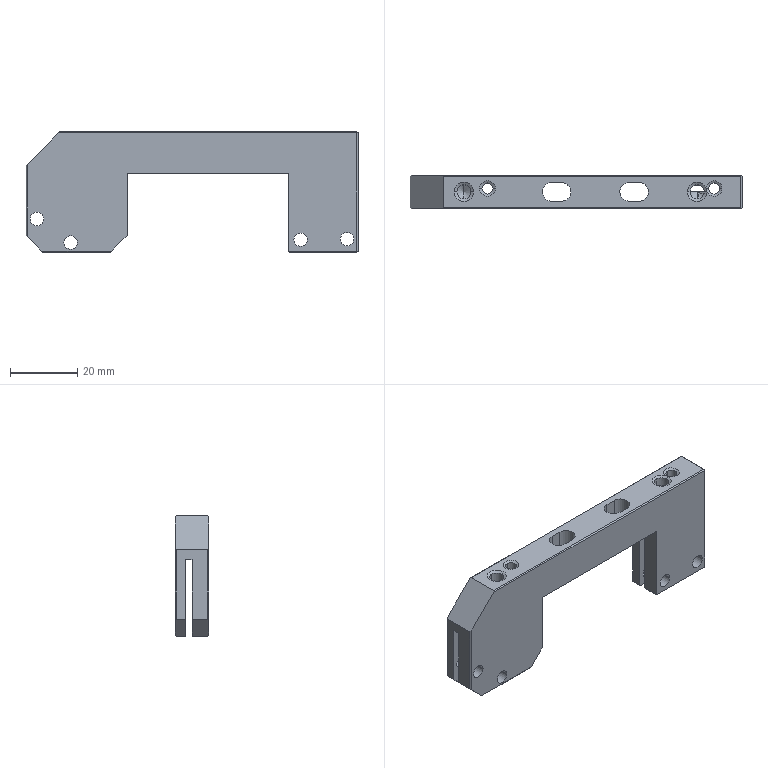Part | NX | 1 solid | 101 faces | box 98.5 x 10 x 35.7 mm | volume 18837 mm3 | plane 49 | cylinder 38 | cone 14 | commonest cylinder face diameters 4 x16 3.3 x8 4.2 x8 5.5 x6